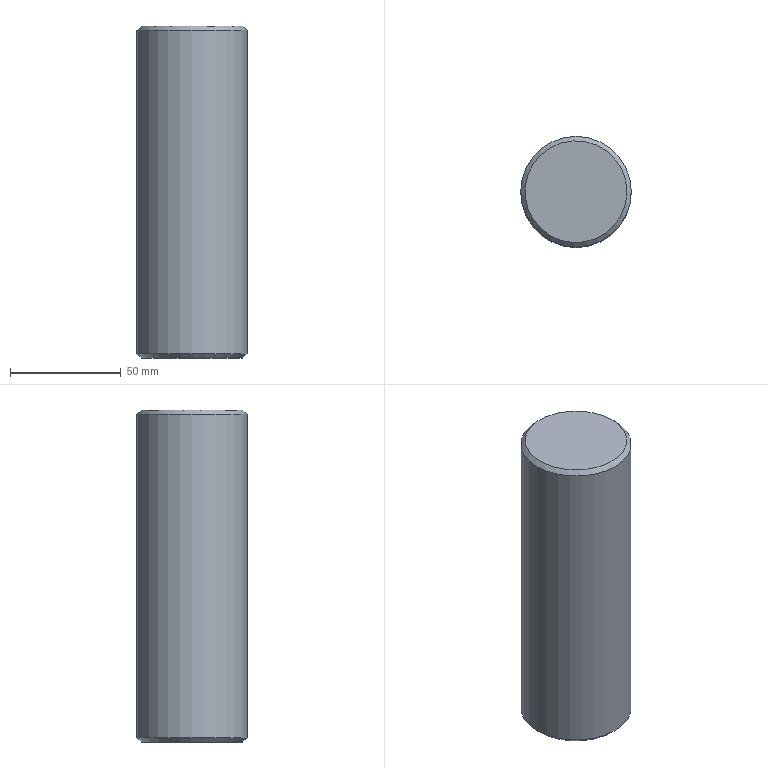Part | STEP file | P011002NM12-000 | 1 solid | 73 faces | box 50 x 50 x 150 mm | volume 291723 mm3 | plane 44 | other 14 | cone 8 | cylinder 7 | commonest cylinder face diameters 10.18 x3 10.2 x1 11.8 x1 12 x1 50 x1